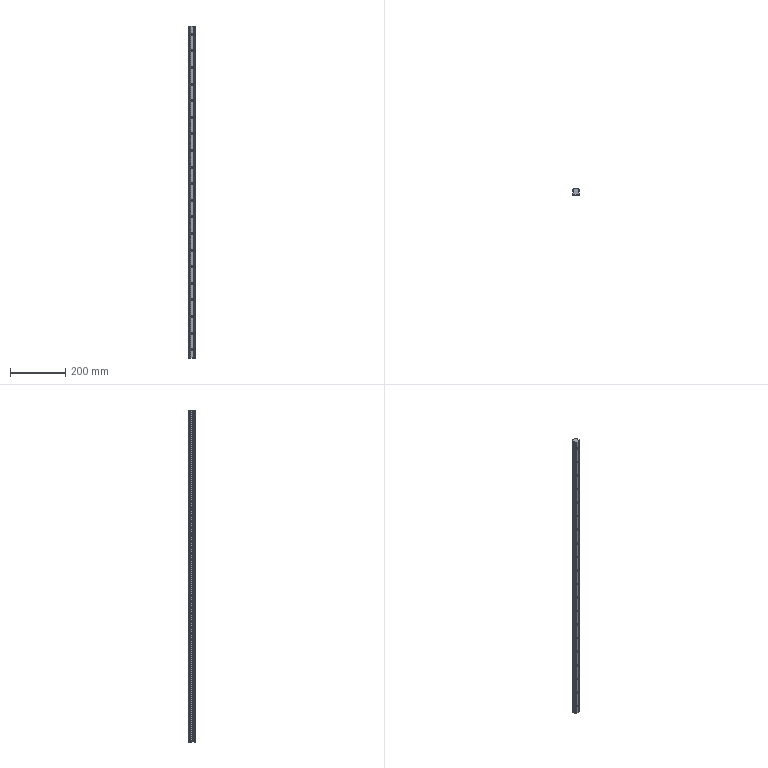Part | SolidWorks | features BaseBody 3 | 1 solid | 134 faces | box 23 x 22 x 1200 mm | volume 500809 mm3 | cylinder 84 | plane 50 | commonest cylinder face diameters 7 x40 11 x40 4.6 x4